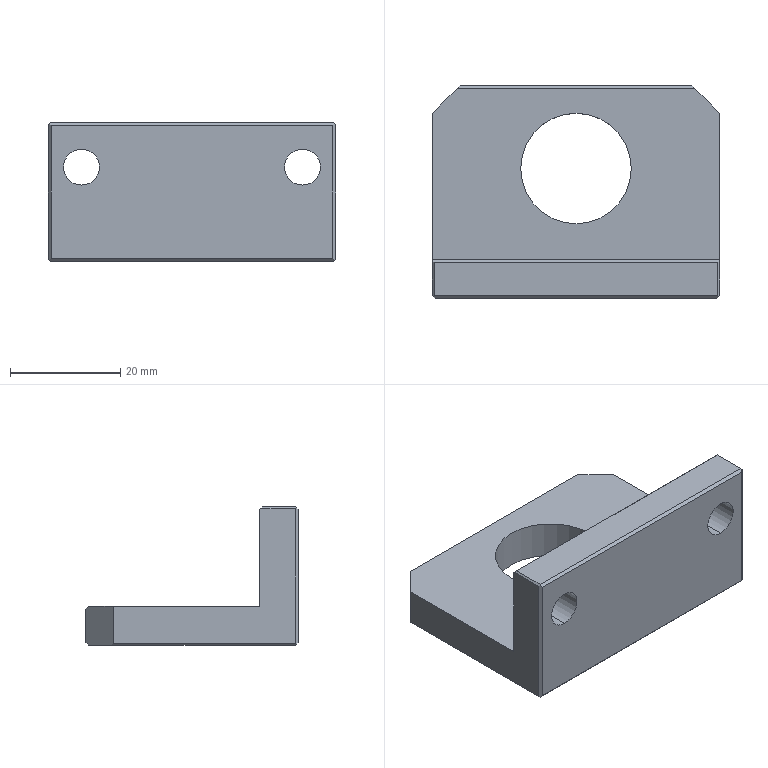Part | STEP file | cylinder seat 2 | 1 solid | 27 faces | box 52 x 38.5 x 25 mm | volume 17688 mm3 | plane 21 | cylinder 6 | commonest cylinder face diameters 6.5 x4 20 x2